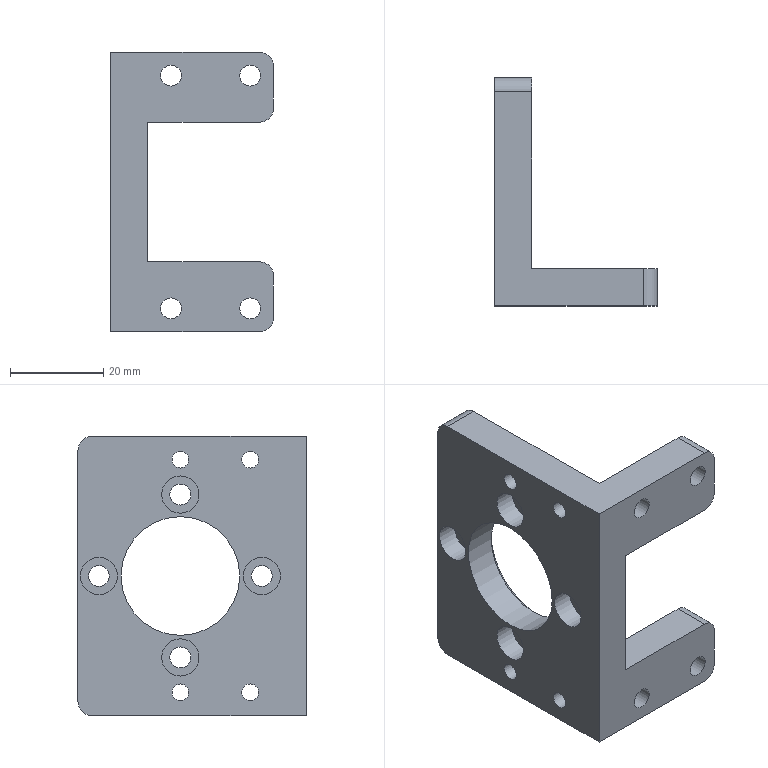Part | 1 solid | 56 faces | box 35 x 49 x 60 mm | volume 22926 mm3 | cylinder 31 | plane 24 | cone 1 | commonest cylinder face diameters 6 x10 4.5 x8 8 x8 3.6 x4 25.5 x1
STEP:
#1=CARTESIAN_POINT('',(4.6,12.,52.));
#2=VERTEX_POINT('',#1);
#3=CARTESIAN_POINT('',(4.6,12.,55.));
#4=DIRECTION('',(1.,0.,0.));
#5=DIRECTION('',(0.,0.,-1.));
#6=AXIS2_PLACEMENT_3D('',#3,#4,#5);
#7=CIRCLE('',#6,3.);
#8=EDGE_CURVE('',#2,#2,#7,.T.);
#9=ORIENTED_EDGE('',*,*,#8,.T.);
#10=EDGE_LOOP('',(#9));
#11=FACE_BOUND('',#10,.T.);
#12=CARTESIAN_POINT('',(4.6,12.,53.2));
#13=VERTEX_POINT('',#12);
#14=CARTESIAN_POINT('',(4.6,12.,55.));
#15=DIRECTION('',(1.,0.,0.));
#16=DIRECTION('',(0.,0.,-1.));
#17=AXIS2_PLACEMENT_3D('',#14,#15,#16);
#18=CIRCLE('',#17,1.8);
#19=EDGE_CURVE('',#13,#13,#18,.T.);
#20=ORIENTED_EDGE('',*,*,#19,.F.);
#21=EDGE_LOOP('',(#20));
#22=FACE_BOUND('',#21,.T.);
#23=CARTESIAN_POINT('',(4.6,13.8,55.));
#24=DIRECTION('',(-1.,0.,0.));
#25=DIRECTION('',(0.,0.,1.));
#26=AXIS2_PLACEMENT_3D('',#23,#24,#25);
#27=PLANE('',#26);
#28=ADVANCED_FACE('',(#11,#22),#27,.F.);
#29=CARTESIAN_POINT('',(4.6,12.,8.));
#30=VERTEX_POINT('',#29);
#31=CARTESIAN_POINT('',(4.6,12.,5.));
#32=DIRECTION('',(1.,0.,0.));
#33=DIRECTION('',(0.,0.,1.));
#34=AXIS2_PLACEMENT_3D('',#31,#32,#33);
#35=CIRCLE('',#34,3.);
#36=EDGE_CURVE('',#30,#30,#35,.T.);
#37=ORIENTED_EDGE('',*,*,#36,.T.);
#38=EDGE_LOOP('',(#37));
#39=FACE_BOUND('',#38,.T.);
#40=CARTESIAN_POINT('',(4.6,12.,6.8));
#41=VERTEX_POINT('',#40);
#42=CARTESIAN_POINT('',(4.6,12.,5.));
#43=DIRECTION('',(1.,0.,0.));
#44=DIRECTION('',(0.,0.,1.));
#45=AXIS2_PLACEMENT_3D('',#42,#43,#44);
#46=CIRCLE('',#45,1.8);
#47=EDGE_CURVE('',#41,#41,#46,.T.);
#48=ORIENTED_EDGE('',*,*,#47,.F.);
#49=EDGE_LOOP('',(#48));
#50=FACE_BOUND('',#49,.T.);
#51=CARTESIAN_POINT('',(4.6,13.8,55.));
#52=DIRECTION('',(-1.,0.,0.));
#53=DIRECTION('',(0.,0.,1.));
#54=AXIS2_PLACEMENT_3D('',#51,#52,#53);
#55=PLANE('',#54);
#56=ADVANCED_FACE('',(#39,#50),#55,.F.);
#57=CARTESIAN_POINT('',(4.6,27.,58.));
#58=VERTEX_POINT('',#57);
#59=CARTESIAN_POINT('',(4.6,27.,55.));
#60=DIRECTION('',(1.,0.,0.));
#61=DIRECTION('',(0.,0.,1.));
#62=AXIS2_PLACEMENT_3D('',#59,#60,#61);
#63=CIRCLE('',#62,3.);
#64=EDGE_CURVE('',#58,#58,#63,.T.);
#65=ORIENTED_EDGE('',*,*,#64,.T.);
#66=EDGE_LOOP('',(#65));
#67=FACE_BOUND('',#66,.T.);
#68=CARTESIAN_POINT('',(4.6,27.,56.8));
#69=VERTEX_POINT('',#68);
#70=CARTESIAN_POINT('',(4.6,27.,55.));
#71=DIRECTION('',(1.,0.,0.));
#72=DIRECTION('',(0.,0.,1.));
#73=AXIS2_PLACEMENT_3D('',#70,#71,#72);
#74=CIRCLE('',#73,1.8);
#75=EDGE_CURVE('',#69,#69,#74,.T.);
#76=ORIENTED_EDGE('',*,*,#75,.F.);
#77=EDGE_LOOP('',(#76));
#78=FACE_BOUND('',#77,.T.);
#79=CARTESIAN_POINT('',(4.6,13.8,55.));
#80=DIRECTION('',(-1.,0.,0.));
#81=DIRECTION('',(0.,0.,1.));
#82=AXIS2_PLACEMENT_3D('',#79,#80,#81);
#83=PLANE('',#82);
#84=ADVANCED_FACE('',(#67,#78),#83,.F.);
#85=CARTESIAN_POINT('',(4.6,27.,8.));
#86=VERTEX_POINT('',#85);
#87=CARTESIAN_POINT('',(4.6,27.,5.));
#88=DIRECTION('',(1.,0.,0.));
#89=DIRECTION('',(0.,0.,1.));
#90=AXIS2_PLACEMENT_3D('',#87,#88,#89);
#91=CIRCLE('',#90,3.);
#92=EDGE_CURVE('',#86,#86,#91,.T.);
#93=ORIENTED_EDGE('',*,*,#92,.T.);
#94=EDGE_LOOP('',(#93));
#95=FACE_BOUND('',#94,.T.);
#96=CARTESIAN_POINT('',(4.6,27.,6.8));
#97=VERTEX_POINT('',#96);
#98=CARTESIAN_POINT('',(4.6,27.,5.));
#99=DIRECTION('',(1.,0.,0.));
#100=DIRECTION('',(0.,0.,1.));
#101=AXIS2_PLACEMENT_3D('',#98,#99,#100);
#102=CIRCLE('',#101,1.8);
#103=EDGE_CURVE('',#97,#97,#102,.T.);
#104=ORIENTED_EDGE('',*,*,#103,.F.);
#105=EDGE_LOOP('',(#104));
#106=FACE_BOUND('',#105,.T.);
#107=CARTESIAN_POINT('',(4.6,13.8,55.));
#108=DIRECTION('',(-1.,0.,0.));
#109=DIRECTION('',(0.,0.,1.));
#110=AXIS2_PLACEMENT_3D('',#107,#108,#109);
#111=PLANE('',#110);
#112=ADVANCED_FACE('',(#95,#106),#111,.F.);
#113=CARTESIAN_POINT('',(13.,3.4,51.));
#114=VERTEX_POINT('',#113);
#115=CARTESIAN_POINT('',(13.,3.4,55.));
#116=DIRECTION('',(0.,1.,0.));
#117=DIRECTION('',(0.,0.,-1.));
#118=AXIS2_PLACEMENT_3D('',#115,#116,#117);
#119=CIRCLE('',#118,4.);
#120=EDGE_CURVE('',#114,#114,#119,.T.);
#121=ORIENTED_EDGE('',*,*,#120,.T.);
#122=EDGE_LOOP('',(#121));
#123=FACE_BOUND('',#122,.T.);
#124=CARTESIAN_POINT('',(13.,3.4,52.75));
#125=VERTEX_POINT('',#124);
#126=CARTESIAN_POINT('',(13.,3.4,55.));
#127=DIRECTION('',(0.,1.,0.));
#128=DIRECTION('',(0.,0.,-1.));
#129=AXIS2_PLACEMENT_3D('',#126,#127,#128);
#130=CIRCLE('',#129,2.25);
#131=EDGE_CURVE('',#125,#125,#130,.T.);
#132=ORIENTED_EDGE('',*,*,#131,.F.);
#133=EDGE_LOOP('',(#132));
#134=FACE_BOUND('',#133,.T.);
#135=CARTESIAN_POINT('',(32.25,3.4,5.));
#136=DIRECTION('',(0.,-1.,0.));
#137=DIRECTION('',(0.,0.,-1.));
#138=AXIS2_PLACEMENT_3D('',#135,#136,#137);
#139=PLANE('',#138);
#140=ADVANCED_FACE('',(#123,#134),#139,.F.);
#141=CARTESIAN_POINT('',(30.,3.4,51.));
#142=VERTEX_POINT('',#141);
#143=CARTESIAN_POINT('',(30.,3.4,55.));
#144=DIRECTION('',(0.,1.,0.));
#145=DIRECTION('',(0.,0.,-1.));
#146=AXIS2_PLACEMENT_3D('',#143,#144,#145);
#147=CIRCLE('',#146,4.);
#148=EDGE_CURVE('',#142,#142,#147,.T.);
#149=ORIENTED_EDGE('',*,*,#148,.T.);
#150=EDGE_LOOP('',(#149));
#151=FACE_BOUND('',#150,.T.);
#152=CARTESIAN_POINT('',(30.,3.4,52.75));
#153=VERTEX_POINT('',#152);
#154=CARTESIAN_POINT('',(30.,3.4,55.));
#155=DIRECTION('',(0.,1.,0.));
#156=DIRECTION('',(0.,0.,-1.));
#157=AXIS2_PLACEMENT_3D('',#154,#155,#156);
#158=CIRCLE('',#157,2.25);
#159=EDGE_CURVE('',#153,#153,#158,.T.);
#160=ORIENTED_EDGE('',*,*,#159,.F.);
#161=EDGE_LOOP('',(#160));
#162=FACE_BOUND('',#161,.T.);
#163=CARTESIAN_POINT('',(32.25,3.4,5.));
#164=DIRECTION('',(0.,-1.,0.));
#165=DIRECTION('',(0.,0.,-1.));
#166=AXIS2_PLACEMENT_3D('',#163,#164,#165);
#167=PLANE('',#166);
#168=ADVANCED_FACE('',(#151,#162),#167,.F.);
#169=CARTESIAN_POINT('',(13.,3.4,1.));
#170=VERTEX_POINT('',#169);
#171=CARTESIAN_POINT('',(13.,3.4,5.));
#172=DIRECTION('',(0.,1.,0.));
#173=DIRECTION('',(0.,0.,-1.));
#174=AXIS2_PLACEMENT_3D('',#171,#172,#173);
#175=CIRCLE('',#174,4.);
#176=EDGE_CURVE('',#170,#170,#175,.T.);
#177=ORIENTED_EDGE('',*,*,#176,.T.);
#178=EDGE_LOOP('',(#177));
#179=FACE_BOUND('',#178,.T.);
#180=CARTESIAN_POINT('',(13.,3.4,2.75));
#181=VERTEX_POINT('',#180);
#182=CARTESIAN_POINT('',(13.,3.4,5.));
#183=DIRECTION('',(0.,1.,0.));
#184=DIRECTION('',(0.,0.,-1.));
#185=AXIS2_PLACEMENT_3D('',#182,#183,#184);
#186=CIRCLE('',#185,2.25);
#187=EDGE_CURVE('',#181,#181,#186,.T.);
#188=ORIENTED_EDGE('',*,*,#187,.F.);
#189=EDGE_LOOP('',(#188));
#190=FACE_BOUND('',#189,.T.);
#191=CARTESIAN_POINT('',(32.25,3.4,5.));
#192=DIRECTION('',(0.,-1.,0.));
#193=DIRECTION('',(0.,0.,-1.));
#194=AXIS2_PLACEMENT_3D('',#191,#192,#193);
#195=PLANE('',#194);
#196=ADVANCED_FACE('',(#179,#190),#195,.F.);
#197=CARTESIAN_POINT('',(30.,3.4,9.));
#198=VERTEX_POINT('',#197);
#199=CARTESIAN_POINT('',(30.,3.4,5.));
#200=DIRECTION('',(0.,1.,0.));
#201=DIRECTION('',(0.,0.,1.));
#202=AXIS2_PLACEMENT_3D('',#199,#200,#201);
#203=CIRCLE('',#202,4.);
#204=EDGE_CURVE('',#198,#198,#203,.T.);
#205=ORIENTED_EDGE('',*,*,#204,.T.);
#206=EDGE_LOOP('',(#205));
#207=FACE_BOUND('',#206,.T.);
#208=CARTESIAN_POINT('',(30.,3.4,7.25));
#209=VERTEX_POINT('',#208);
#210=CARTESIAN_POINT('',(30.,3.4,5.));
#211=DIRECTION('',(0.,1.,0.));
#212=DIRECTION('',(0.,0.,1.));
#213=AXIS2_PLACEMENT_3D('',#210,#211,#212);
#214=CIRCLE('',#213,2.25);
#215=EDGE_CURVE('',#209,#209,#214,.T.);
#216=ORIENTED_EDGE('',*,*,#215,.F.);
#217=EDGE_LOOP('',(#216));
#218=FACE_BOUND('',#217,.T.);
#219=CARTESIAN_POINT('',(32.25,3.4,5.));
#220=DIRECTION('',(0.,-1.,0.));
#221=DIRECTION('',(0.,0.,-1.));
#222=AXIS2_PLACEMENT_3D('',#219,#220,#221);
#223=PLANE('',#222);
#224=ADVANCED_FACE('',(#207,#218),#223,.F.);
#225=CARTESIAN_POINT('',(35.,0.,12.));
#226=VERTEX_POINT('',#225);
#227=CARTESIAN_POINT('',(32.,0.,15.));
#228=VERTEX_POINT('',#227);
#229=CARTESIAN_POINT('',(32.,0.,12.));
#230=DIRECTION('',(0.,-1.,0.));
#231=DIRECTION('',(0.,0.,1.));
#232=AXIS2_PLACEMENT_3D('',#229,#230,#231);
#233=CIRCLE('',#232,3.);
#234=EDGE_CURVE('',#226,#228,#233,.T.);
#235=ORIENTED_EDGE('',*,*,#234,.F.);
#236=CARTESIAN_POINT('',(35.,8.,12.));
#237=VERTEX_POINT('',#236);
#238=CARTESIAN_POINT('',(35.,0.,12.));
#239=DIRECTION('',(0.,-1.,0.));
#240=VECTOR('',#239,1000.);
#241=LINE('',#238,#240);
#242=EDGE_CURVE('',#237,#226,#241,.T.);
#243=ORIENTED_EDGE('',*,*,#242,.F.);
#244=CARTESIAN_POINT('',(32.,8.,15.));
#245=VERTEX_POINT('',#244);
#246=CARTESIAN_POINT('',(32.,8.,12.));
#247=DIRECTION('',(0.,1.,0.));
#248=DIRECTION('',(1.,0.,0.));
#249=AXIS2_PLACEMENT_3D('',#246,#247,#248);
#250=CIRCLE('',#249,3.);
#251=EDGE_CURVE('',#245,#237,#250,.T.);
#252=ORIENTED_EDGE('',*,*,#251,.F.);
#253=CARTESIAN_POINT('',(32.,-2.,15.));
#254=DIRECTION('',(0.,1.,0.));
#255=VECTOR('',#254,1000.);
#256=LINE('',#253,#255);
#257=EDGE_CURVE('',#228,#245,#256,.T.);
#258=ORIENTED_EDGE('',*,*,#257,.F.);
#259=EDGE_LOOP('',(#235,#243,#252,#258));
#260=FACE_BOUND('',#259,.T.);
#261=CARTESIAN_POINT('',(32.,-2.,12.));
#262=DIRECTION('',(0.,1.,0.));
#263=DIRECTION('',(0.,0.,1.));
#264=AXIS2_PLACEMENT_3D('',#261,#262,#263);
#265=CYLINDRICAL_SURFACE('',#264,3.);
#266=ADVANCED_FACE('',(#260),#265,.T.);
#267=CARTESIAN_POINT('',(32.,0.,0.));
#268=VERTEX_POINT('',#267);
#269=CARTESIAN_POINT('',(35.,0.,3.));
#270=VERTEX_POINT('',#269);
#271=CARTESIAN_POINT('',(32.,0.,3.));
#272=DIRECTION('',(0.,-1.,0.));
#273=DIRECTION('',(0.,0.,1.));
#274=AXIS2_PLACEMENT_3D('',#271,#272,#273);
#275=CIRCLE('',#274,3.);
#276=EDGE_CURVE('',#268,#270,#275,.T.);
#277=ORIENTED_EDGE('',*,*,#276,.F.);
#278=CARTESIAN_POINT('',(32.,8.,0.));
#279=VERTEX_POINT('',#278);
#280=CARTESIAN_POINT('',(32.,0.,0.));
#281=DIRECTION('',(0.,-1.,0.));
#282=VECTOR('',#281,1000.);
#283=LINE('',#280,#282);
#284=EDGE_CURVE('',#279,#268,#283,.T.);
#285=ORIENTED_EDGE('',*,*,#284,.F.);
#286=CARTESIAN_POINT('',(35.,8.,3.));
#287=VERTEX_POINT('',#286);
#288=CARTESIAN_POINT('',(32.,8.,3.));
#289=DIRECTION('',(0.,1.,0.));
#290=DIRECTION('',(1.,0.,0.));
#291=AXIS2_PLACEMENT_3D('',#288,#289,#290);
#292=CIRCLE('',#291,3.);
#293=EDGE_CURVE('',#287,#279,#292,.T.);
#294=ORIENTED_EDGE('',*,*,#293,.F.);
#295=CARTESIAN_POINT('',(35.,0.,3.));
#296=DIRECTION('',(0.,1.,0.));
#297=VECTOR('',#296,1000.);
#298=LINE('',#295,#297);
#299=EDGE_CURVE('',#270,#287,#298,.T.);
#300=ORIENTED_EDGE('',*,*,#299,.F.);
#301=EDGE_LOOP('',(#277,#285,#294,#300));
#302=FACE_BOUND('',#301,.T.);
#303=CARTESIAN_POINT('',(32.,0.,3.));
#304=DIRECTION('',(0.,1.,0.));
#305=DIRECTION('',(0.,0.,1.));
#306=AXIS2_PLACEMENT_3D('',#303,#304,#305);
#307=CYLINDRICAL_SURFACE('',#306,3.);
#308=ADVANCED_FACE('',(#302),#307,.T.);
#309=CARTESIAN_POINT('',(32.,0.,45.));
#310=VERTEX_POINT('',#309);
#311=CARTESIAN_POINT('',(35.,0.,48.));
#312=VERTEX_POINT('',#311);
#313=CARTESIAN_POINT('',(32.,0.,48.));
#314=DIRECTION('',(0.,-1.,0.));
#315=DIRECTION('',(0.,0.,1.));
#316=AXIS2_PLACEMENT_3D('',#313,#314,#315);
#317=CIRCLE('',#316,3.);
#318=EDGE_CURVE('',#310,#312,#317,.T.);
#319=ORIENTED_EDGE('',*,*,#318,.F.);
#320=CARTESIAN_POINT('',(32.,8.,45.));
#321=VERTEX_POINT('',#320);
#322=CARTESIAN_POINT('',(32.,-2.,45.));
#323=DIRECTION('',(0.,-1.,0.));
#324=VECTOR('',#323,1000.);
#325=LINE('',#322,#324);
#326=EDGE_CURVE('',#321,#310,#325,.T.);
#327=ORIENTED_EDGE('',*,*,#326,.F.);
#328=CARTESIAN_POINT('',(35.,8.,48.));
#329=VERTEX_POINT('',#328);
#330=CARTESIAN_POINT('',(32.,8.,48.));
#331=DIRECTION('',(0.,1.,0.));
#332=DIRECTION('',(1.,0.,0.));
#333=AXIS2_PLACEMENT_3D('',#330,#331,#332);
#334=CIRCLE('',#333,3.);
#335=EDGE_CURVE('',#329,#321,#334,.T.);
#336=ORIENTED_EDGE('',*,*,#335,.F.);
#337=CARTESIAN_POINT('',(35.,0.,48.));
#338=DIRECTION('',(0.,1.,0.));
#339=VECTOR('',#338,1000.);
#340=LINE('',#337,#339);
#341=EDGE_CURVE('',#312,#329,#340,.T.);
#342=ORIENTED_EDGE('',*,*,#341,.F.);
#343=EDGE_LOOP('',(#319,#327,#336,#342));
#344=FACE_BOUND('',#343,.T.);
#345=CARTESIAN_POINT('',(32.,0.,48.));
#346=DIRECTION('',(0.,1.,0.));
#347=DIRECTION('',(0.,0.,1.));
#348=AXIS2_PLACEMENT_3D('',#345,#346,#347);
#349=CYLINDRICAL_SURFACE('',#348,3.);
#350=ADVANCED_FACE('',(#344),#349,.T.);
#351=CARTESIAN_POINT('',(35.,0.,57.));
#352=VERTEX_POINT('',#351);
#353=CARTESIAN_POINT('',(32.,0.,60.));
#354=VERTEX_POINT('',#353);
#355=CARTESIAN_POINT('',(32.,0.,57.));
#356=DIRECTION('',(0.,-1.,0.));
#357=DIRECTION('',(0.,0.,1.));
#358=AXIS2_PLACEMENT_3D('',#355,#356,#357);
#359=CIRCLE('',#358,3.);
#360=EDGE_CURVE('',#352,#354,#359,.T.);
#361=ORIENTED_EDGE('',*,*,#360,.F.);
#362=CARTESIAN_POINT('',(35.,8.,57.));
#363=VERTEX_POINT('',#362);
#364=CARTESIAN_POINT('',(35.,0.,57.));
#365=DIRECTION('',(0.,-1.,0.));
#366=VECTOR('',#365,1000.);
#367=LINE('',#364,#366);
#368=EDGE_CURVE('',#363,#352,#367,.T.);
#369=ORIENTED_EDGE('',*,*,#368,.F.);
#370=CARTESIAN_POINT('',(32.,8.,60.));
#371=VERTEX_POINT('',#370);
#372=CARTESIAN_POINT('',(32.,8.,57.));
#373=DIRECTION('',(0.,1.,0.));
#374=DIRECTION('',(1.,0.,0.));
#375=AXIS2_PLACEMENT_3D('',#372,#373,#374);
#376=CIRCLE('',#375,3.);
#377=EDGE_CURVE('',#371,#363,#376,.T.);
#378=ORIENTED_EDGE('',*,*,#377,.F.);
#379=CARTESIAN_POINT('',(32.,8.,60.));
#380=DIRECTION('',(0.,1.,0.));
#381=VECTOR('',#380,1000.);
#382=LINE('',#379,#381);
#383=EDGE_CURVE('',#354,#371,#382,.T.);
#384=ORIENTED_EDGE('',*,*,#383,.F.);
#385=EDGE_LOOP('',(#361,#369,#378,#384));
#386=FACE_BOUND('',#385,.T.);
#387=CARTESIAN_POINT('',(32.,0.,57.));
#388=DIRECTION('',(0.,-1.,0.));
#389=DIRECTION('',(0.,0.,-1.));
#390=AXIS2_PLACEMENT_3D('',#387,#388,#389);
#391=CYLINDRICAL_SURFACE('',#390,3.);
#392=ADVANCED_FACE('',(#386),#391,.T.);
#393=CARTESIAN_POINT('',(8.,49.,57.));
#394=VERTEX_POINT('',#393);
#395=CARTESIAN_POINT('',(8.,46.,60.));
#396=VERTEX_POINT('',#395);
#397=CARTESIAN_POINT('',(8.,46.,57.));
#398=DIRECTION('',(1.,0.,0.));
#399=DIRECTION('',(0.,0.,1.));
#400=AXIS2_PLACEMENT_3D('',#397,#398,#399);
#401=CIRCLE('',#400,3.);
#402=EDGE_CURVE('',#394,#396,#401,.T.);
#403=ORIENTED_EDGE('',*,*,#402,.F.);
#404=CARTESIAN_POINT('',(0.,49.,57.));
#405=VERTEX_POINT('',#404);
#406=CARTESIAN_POINT('',(8.,49.,57.));
#407=DIRECTION('',(1.,0.,0.));
#408=VECTOR('',#407,1000.);
#409=LINE('',#406,#408);
#410=EDGE_CURVE('',#405,#394,#409,.T.);
#411=ORIENTED_EDGE('',*,*,#410,.F.);
#412=CARTESIAN_POINT('',(0.,46.,60.));
#413=VERTEX_POINT('',#412);
#414=CARTESIAN_POINT('',(0.,46.,57.));
#415=DIRECTION('',(-1.,0.,0.));
#416=DIRECTION('',(0.,0.,-1.));
#417=AXIS2_PLACEMENT_3D('',#414,#415,#416);
#418=CIRCLE('',#417,3.);
#419=EDGE_CURVE('',#413,#405,#418,.T.);
#420=ORIENTED_EDGE('',*,*,#419,.F.);
#421=CARTESIAN_POINT('',(0.,46.,60.));
#422=DIRECTION('',(-1.,0.,0.));
#423=VECTOR('',#422,1000.);
#424=LINE('',#421,#423);
#425=EDGE_CURVE('',#396,#413,#424,.T.);
#426=ORIENTED_EDGE('',*,*,#425,.F.);
#427=EDGE_LOOP('',(#403,#411,#420,#426));
#428=FACE_BOUND('',#427,.T.);
#429=CARTESIAN_POINT('',(0.,46.,57.));
#430=DIRECTION('',(1.,0.,0.));
#431=DIRECTION('',(0.,0.,-1.));
#432=AXIS2_PLACEMENT_3D('',#429,#430,#431);
#433=CYLINDRICAL_SURFACE('',#432,3.);
#434=ADVANCED_FACE('',(#428),#433,.T.);
#435=CARTESIAN_POINT('',(8.,46.,0.));
#436=VERTEX_POINT('',#435);
#437=CARTESIAN_POINT('',(8.,49.,3.));
#438=VERTEX_POINT('',#437);
#439=CARTESIAN_POINT('',(8.,46.,3.));
#440=DIRECTION('',(1.,0.,0.));
#441=DIRECTION('',(0.,0.,1.));
#442=AXIS2_PLACEMENT_3D('',#439,#440,#441);
#443=CIRCLE('',#442,3.);
#444=EDGE_CURVE('',#436,#438,#443,.T.);
#445=ORIENTED_EDGE('',*,*,#444,.F.);
#446=CARTESIAN_POINT('',(0.,46.,0.));
#447=VERTEX_POINT('',#446);
#448=CARTESIAN_POINT('',(0.,46.,0.));
#449=DIRECTION('',(1.,0.,0.));
#450=VECTOR('',#449,1000.);
#451=LINE('',#448,#450);
#452=EDGE_CURVE('',#447,#436,#451,.T.);
#453=ORIENTED_EDGE('',*,*,#452,.F.);
#454=CARTESIAN_POINT('',(0.,49.,3.));
#455=VERTEX_POINT('',#454);
#456=CARTESIAN_POINT('',(0.,46.,3.));
#457=DIRECTION('',(-1.,0.,0.));
#458=DIRECTION('',(0.,0.,-1.));
#459=AXIS2_PLACEMENT_3D('',#456,#457,#458);
#460=CIRCLE('',#459,3.);
#461=EDGE_CURVE('',#455,#447,#460,.T.);
#462=ORIENTED_EDGE('',*,*,#461,.F.);
#463=CARTESIAN_POINT('',(8.,49.,3.));
#464=DIRECTION('',(-1.,0.,0.));
#465=VECTOR('',#464,1000.);
#466=LINE('',#463,#465);
#467=EDGE_CURVE('',#438,#455,#466,.T.);
#468=ORIENTED_EDGE('',*,*,#467,.F.);
#469=EDGE_LOOP('',(#445,#453,#462,#468));
#470=FACE_BOUND('',#469,.T.);
#471=CARTESIAN_POINT('',(8.,46.,3.));
#472=DIRECTION('',(-1.,0.,0.));
#473=DIRECTION('',(0.,0.,1.));
#474=AXIS2_PLACEMENT_3D('',#471,#472,#473);
#475=CYLINDRICAL_SURFACE('',#474,3.);
#476=ADVANCED_FACE('',(#470),#475,.T.);
#477=CARTESIAN_POINT('',(8.,0.,15.));
#478=VERTEX_POINT('',#477);
#479=CARTESIAN_POINT('',(0.,0.,15.));
#480=DIRECTION('',(-1.,0.,0.));
#481=VECTOR('',#480,1000.);
#482=LINE('',#479,#481);
#483=EDGE_CURVE('',#228,#478,#482,.T.);
#484=ORIENTED_EDGE('',*,*,#483,.F.);
#485=ORIENTED_EDGE('',*,*,#257,.T.);
#486=CARTESIAN_POINT('',(8.,8.,15.));
#487=VERTEX_POINT('',#486);
#488=CARTESIAN_POINT('',(8.,8.,15.));
#489=DIRECTION('',(-1.,0.,0.));
#490=VECTOR('',#489,1000.);
#491=LINE('',#488,#490);
#492=EDGE_CURVE('',#245,#487,#491,.T.);
#493=ORIENTED_EDGE('',*,*,#492,.T.);
#494=CARTESIAN_POINT('',(8.,-2.,15.));
#495=DIRECTION('',(0.,1.,0.));
#496=VECTOR('',#495,1000.);
#497=LINE('',#494,#496);
#498=EDGE_CURVE('',#478,#487,#497,.T.);
#499=ORIENTED_EDGE('',*,*,#498,.F.);
#500=EDGE_LOOP('',(#484,#485,#493,#499));
#501=FACE_BOUND('',#500,.T.);
#502=CARTESIAN_POINT('',(8.,-2.,15.));
#503=DIRECTION('',(0.,0.,-1.));
#504=DIRECTION('',(-1.,0.,0.));
#505=AXIS2_PLACEMENT_3D('',#502,#503,#504);
#506=PLANE('',#505);
#507=ADVANCED_FACE('',(#501),#506,.F.);
#508=CARTESIAN_POINT('',(8.,8.,45.));
#509=VERTEX_POINT('',#508);
#510=CARTESIAN_POINT('',(8.,8.,45.));
#511=DIRECTION('',(1.,0.,0.));
#512=VECTOR('',#511,1000.);
#513=LINE('',#510,#512);
#514=EDGE_CURVE('',#509,#321,#513,.T.);
#515=ORIENTED_EDGE('',*,*,#514,.T.);
#516=ORIENTED_EDGE('',*,*,#326,.T.);
#517=CARTESIAN_POINT('',(8.,0.,45.));
#518=VERTEX_POINT('',#517);
#519=CARTESIAN_POINT('',(0.,0.,45.));
#520=DIRECTION('',(1.,0.,0.));
#521=VECTOR('',#520,1000.);
#522=LINE('',#519,#521);
#523=EDGE_CURVE('',#518,#310,#522,.T.);
#524=ORIENTED_EDGE('',*,*,#523,.F.);
#525=CARTESIAN_POINT('',(8.,-2.,45.));
#526=DIRECTION('',(0.,1.,0.));
#527=VECTOR('',#526,1000.);
#528=LINE('',#525,#527);
#529=EDGE_CURVE('',#518,#509,#528,.T.);
#530=ORIENTED_EDGE('',*,*,#529,.T.);
#531=EDGE_LOOP('',(#515,#516,#524,#530));
#532=FACE_BOUND('',#531,.T.);
#533=CARTESIAN_POINT('',(8.,-2.,45.));
#534=DIRECTION('',(0.,0.,1.));
#535=DIRECTION('',(1.,0.,0.));
#536=AXIS2_PLACEMENT_3D('',#533,#534,#535);
#537=PLANE('',#536);
#538=ADVANCED_FACE('',(#532),#537,.F.);
#539=CARTESIAN_POINT('',(4.6,27.,51.5));
#540=VERTEX_POINT('',#539);
#541=CARTESIAN_POINT('',(4.6,27.,47.5));
#542=DIRECTION('',(-1.,0.,0.));
#543=DIRECTION('',(0.,0.,1.));
#544=AXIS2_PLACEMENT_3D('',#541,#542,#543);
#545=CIRCLE('',#544,4.);
#546=EDGE_CURVE('',#540,#540,#545,.T.);
#547=ORIENTED_EDGE('',*,*,#546,.T.);
#548=EDGE_LOOP('',(#547));
#549=FACE_BOUND('',#548,.T.);
#550=CARTESIAN_POINT('',(4.6,27.,49.75));
#551=VERTEX_POINT('',#550);
#552=CARTESIAN_POINT('',(4.6,27.,47.5));
#553=DIRECTION('',(-1.,0.,0.));
#554=DIRECTION('',(0.,0.,1.));
#555=AXIS2_PLACEMENT_3D('',#552,#553,#554);
#556=CIRCLE('',#555,2.25);
#557=EDGE_CURVE('',#551,#551,#556,.T.);
#558=ORIENTED_EDGE('',*,*,#557,.F.);
#559=EDGE_LOOP('',(#558));
#560=FACE_BOUND('',#559,.T.);
#561=CARTESIAN_POINT('',(4.6,13.8,55.));
#562=DIRECTION('',(-1.,0.,0.));
#563=DIRECTION('',(0.,0.,1.));
#564=AXIS2_PLACEMENT_3D('',#561,#562,#563);
#565=PLANE('',#564);
#566=ADVANCED_FACE('',(#549,#560),#565,.T.);
#567=CARTESIAN_POINT('',(4.6,27.,16.5));
#568=VERTEX_POINT('',#567);
#569=CARTESIAN_POINT('',(4.6,27.,12.5));
#570=DIRECTION('',(-1.,0.,0.));
#571=DIRECTION('',(0.,0.,1.));
#572=AXIS2_PLACEMENT_3D('',#569,#570,#571);
#573=CIRCLE('',#572,4.);
#574=EDGE_CURVE('',#568,#568,#573,.T.);
#575=ORIENTED_EDGE('',*,*,#574,.T.);
#576=EDGE_LOOP('',(#575));
#577=FACE_BOUND('',#576,.T.);
#578=CARTESIAN_POINT('',(4.6,27.,14.75));
#579=VERTEX_POINT('',#578);
#580=CARTESIAN_POINT('',(4.6,27.,12.5));
#581=DIRECTION('',(-1.,0.,0.));
#582=DIRECTION('',(0.,0.,1.));
#583=AXIS2_PLACEMENT_3D('',#580,#581,#582);
#584=CIRCLE('',#583,2.25);
#585=EDGE_CURVE('',#579,#579,#584,.T.);
#586=ORIENTED_EDGE('',*,*,#585,.F.);
#587=EDGE_LOOP('',(#586));
#588=FACE_BOUND('',#587,.T.);
#589=CARTESIAN_POINT('',(4.6,13.8,55.));
#590=DIRECTION('',(-1.,0.,0.));
#591=DIRECTION('',(0.,0.,1.));
#592=AXIS2_PLACEMENT_3D('',#589,#590,#591);
#593=PLANE('',#592);
#594=ADVANCED_FACE('',(#577,#588),#593,.T.);
#595=CARTESIAN_POINT('',(4.6,44.5,34.));
#596=VERTEX_POINT('',#595);
#597=CARTESIAN_POINT('',(4.6,44.5,30.));
#598=DIRECTION('',(-1.,0.,0.));
#599=DIRECTION('',(0.,0.,1.));
#600=AXIS2_PLACEMENT_3D('',#597,#598,#599);
#601=CIRCLE('',#600,4.);
#602=EDGE_CURVE('',#596,#596,#601,.T.);
#603=ORIENTED_EDGE('',*,*,#602,.T.);
#604=EDGE_LOOP('',(#603));
#605=FACE_BOUND('',#604,.T.);
#606=CARTESIAN_POINT('',(4.6,44.5,32.25));
#607=VERTEX_POINT('',#606);
#608=CARTESIAN_POINT('',(4.6,44.5,30.));
#609=DIRECTION('',(-1.,0.,0.));
#610=DIRECTION('',(0.,0.,1.));
#611=AXIS2_PLACEMENT_3D('',#608,#609,#610);
#612=CIRCLE('',#611,2.25);
#613=EDGE_CURVE('',#607,#607,#612,.T.);
#614=ORIENTED_EDGE('',*,*,#613,.F.);
#615=EDGE_LOOP('',(#614));
#616=FACE_BOUND('',#615,.T.);
#617=CARTESIAN_POINT('',(4.6,13.8,55.));
#618=DIRECTION('',(-1.,0.,0.));
#619=DIRECTION('',(0.,0.,1.));
#620=AXIS2_PLACEMENT_3D('',#617,#618,#619);
#621=PLANE('',#620);
#622=ADVANCED_FACE('',(#605,#616),#621,.T.);
#623=CARTESIAN_POINT('',(4.6,9.5,34.));
#624=VERTEX_POINT('',#623);
#625=CARTESIAN_POINT('',(4.6,9.5,30.));
#626=DIRECTION('',(-1.,0.,0.));
#627=DIRECTION('',(0.,0.,1.));
#628=AXIS2_PLACEMENT_3D('',#625,#626,#627);
#629=CIRCLE('',#628,4.);
#630=EDGE_CURVE('',#624,#624,#629,.T.);
#631=ORIENTED_EDGE('',*,*,#630,.T.);
#632=EDGE_LOOP('',(#631));
#633=FACE_BOUND('',#632,.T.);
#634=CARTESIAN_POINT('',(4.6,9.5,32.25));
#635=VERTEX_POINT('',#634);
#636=CARTESIAN_POINT('',(4.6,9.5,30.));
#637=DIRECTION('',(-1.,0.,0.));
#638=DIRECTION('',(0.,0.,1.));
#639=AXIS2_PLACEMENT_3D('',#636,#637,#638);
#640=CIRCLE('',#639,2.25);
#641=EDGE_CURVE('',#635,#635,#640,.T.);
#642=ORIENTED_EDGE('',*,*,#641,.F.);
#643=EDGE_LOOP('',(#642));
#644=FACE_BOUND('',#643,.T.);
#645=CARTESIAN_POINT('',(4.6,13.8,55.));
#646=DIRECTION('',(-1.,0.,0.));
#647=DIRECTION('',(0.,0.,1.));
#648=AXIS2_PLACEMENT_3D('',#645,#646,#647);
#649=PLANE('',#648);
#650=ADVANCED_FACE('',(#633,#644),#649,.T.);
#651=CARTESIAN_POINT('',(0.,0.,0.));
#652=VERTEX_POINT('',#651);
#653=CARTESIAN_POINT('',(0.,49.,0.));
#654=DIRECTION('',(0.,-1.,0.));
#655=VECTOR('',#654,1000.);
#656=LINE('',#653,#655);
#657=EDGE_CURVE('',#447,#652,#656,.T.);
#658=ORIENTED_EDGE('',*,*,#657,.F.);
#659=ORIENTED_EDGE('',*,*,#452,.T.);
#660=CARTESIAN_POINT('',(8.,8.,0.));
#661=VERTEX_POINT('',#660);
#662=CARTESIAN_POINT('',(8.,8.,0.));
#663=DIRECTION('',(0.,1.,0.));
#664=VECTOR('',#663,1000.);
#665=LINE('',#662,#664);
#666=EDGE_CURVE('',#661,#436,#665,.T.);
#667=ORIENTED_EDGE('',*,*,#666,.F.);
#668=CARTESIAN_POINT('',(35.,8.,0.));
#669=DIRECTION('',(-1.,0.,0.));
#670=VECTOR('',#669,1000.);
#671=LINE('',#668,#670);
#672=EDGE_CURVE('',#279,#661,#671,.T.);
#673=ORIENTED_EDGE('',*,*,#672,.F.);
#674=ORIENTED_EDGE('',*,*,#284,.T.);
#675=CARTESIAN_POINT('',(0.,0.,0.));
#676=DIRECTION('',(1.,0.,0.));
#677=VECTOR('',#676,1000.);
#678=LINE('',#675,#677);
#679=EDGE_CURVE('',#652,#268,#678,.T.);
#680=ORIENTED_EDGE('',*,*,#679,.F.);
#681=EDGE_LOOP('',(#658,#659,#667,#673,#674,#680));
#682=FACE_BOUND('',#681,.T.);
#683=CARTESIAN_POINT('',(0.,0.,0.));
#684=DIRECTION('',(0.,0.,1.));
#685=DIRECTION('',(1.,0.,0.));
#686=AXIS2_PLACEMENT_3D('',#683,#684,#685);
#687=PLANE('',#686);
#688=ADVANCED_FACE('',(#682),#687,.F.);
#689=CARTESIAN_POINT('',(8.,8.,60.));
#690=VERTEX_POINT('',#689);
#691=CARTESIAN_POINT('',(8.,8.,60.));
#692=DIRECTION('',(0.,1.,0.));
#693=VECTOR('',#692,1000.);
#694=LINE('',#691,#693);
#695=EDGE_CURVE('',#690,#396,#694,.T.);
#696=ORIENTED_EDGE('',*,*,#695,.T.);
#697=ORIENTED_EDGE('',*,*,#425,.T.);
#698=CARTESIAN_POINT('',(0.,0.,60.));
#699=VERTEX_POINT('',#698);
#700=CARTESIAN_POINT('',(0.,49.,60.));
#701=DIRECTION('',(0.,-1.,0.));
#702=VECTOR('',#701,1000.);
#703=LINE('',#700,#702);
#704=EDGE_CURVE('',#413,#699,#703,.T.);
#705=ORIENTED_EDGE('',*,*,#704,.T.);
#706=CARTESIAN_POINT('',(0.,0.,60.));
#707=DIRECTION('',(1.,0.,0.));
#708=VECTOR('',#707,1000.);
#709=LINE('',#706,#708);
#710=EDGE_CURVE('',#699,#354,#709,.T.);
#711=ORIENTED_EDGE('',*,*,#710,.T.);
#712=ORIENTED_EDGE('',*,*,#383,.T.);
#713=CARTESIAN_POINT('',(35.,8.,60.));
#714=DIRECTION('',(-1.,0.,0.));
#715=VECTOR('',#714,1000.);
#716=LINE('',#713,#715);
#717=EDGE_CURVE('',#371,#690,#716,.T.);
#718=ORIENTED_EDGE('',*,*,#717,.T.);
#719=EDGE_LOOP('',(#696,#697,#705,#711,#712,#718));
#720=FACE_BOUND('',#719,.T.);
#721=CARTESIAN_POINT('',(0.,0.,60.));
#722=DIRECTION('',(0.,0.,1.));
#723=DIRECTION('',(1.,0.,0.));
#724=AXIS2_PLACEMENT_3D('',#721,#722,#723);
#725=PLANE('',#724);
#726=ADVANCED_FACE('',(#720),#725,.T.);
#727=CARTESIAN_POINT('',(8.,9.5,32.25));
#728=VERTEX_POINT('',#727);
#729=CARTESIAN_POINT('',(8.,9.5,30.));
#730=DIRECTION('',(-1.,0.,0.));
#731=DIRECTION('',(0.,0.,1.));
#732=AXIS2_PLACEMENT_3D('',#729,#730,#731);
#733=CIRCLE('',#732,2.25);
#734=EDGE_CURVE('',#728,#728,#733,.T.);
#735=ORIENTED_EDGE('',*,*,#734,.T.);
#736=EDGE_LOOP('',(#735));
#737=FACE_BOUND('',#736,.T.);
#738=CARTESIAN_POINT('',(8.,44.5,32.25));
#739=VERTEX_POINT('',#738);
#740=CARTESIAN_POINT('',(8.,44.5,30.));
#741=DIRECTION('',(-1.,0.,0.));
#742=DIRECTION('',(0.,0.,1.));
#743=AXIS2_PLACEMENT_3D('',#740,#741,#742);
#744=CIRCLE('',#743,2.25);
#745=EDGE_CURVE('',#739,#739,#744,.T.);
#746=ORIENTED_EDGE('',*,*,#745,.T.);
#747=EDGE_LOOP('',(#746));
#748=FACE_BOUND('',#747,.T.);
#749=CARTESIAN_POINT('',(8.,27.,14.75));
#750=VERTEX_POINT('',#749);
#751=CARTESIAN_POINT('',(8.,27.,12.5));
#752=DIRECTION('',(-1.,0.,0.));
#753=DIRECTION('',(0.,0.,1.));
#754=AXIS2_PLACEMENT_3D('',#751,#752,#753);
#755=CIRCLE('',#754,2.25);
#756=EDGE_CURVE('',#750,#750,#755,.T.);
#757=ORIENTED_EDGE('',*,*,#756,.T.);
#758=EDGE_LOOP('',(#757));
#759=FACE_BOUND('',#758,.T.);
#760=CARTESIAN_POINT('',(8.,27.,49.75));
#761=VERTEX_POINT('',#760);
#762=CARTESIAN_POINT('',(8.,27.,47.5));
#763=DIRECTION('',(-1.,0.,0.));
#764=DIRECTION('',(0.,0.,1.));
#765=AXIS2_PLACEMENT_3D('',#762,#763,#764);
#766=CIRCLE('',#765,2.25);
#767=EDGE_CURVE('',#761,#761,#766,.T.);
#768=ORIENTED_EDGE('',*,*,#767,.T.);
#769=EDGE_LOOP('',(#768));
#770=FACE_BOUND('',#769,.T.);
#771=CARTESIAN_POINT('',(8.,27.,43.75));
#772=VERTEX_POINT('',#771);
#773=CARTESIAN_POINT('',(8.,27.,30.));
#774=DIRECTION('',(-1.,0.,0.));
#775=DIRECTION('',(0.,0.,1.));
#776=AXIS2_PLACEMENT_3D('',#773,#774,#775);
#777=CIRCLE('',#776,13.75);
#778=EDGE_CURVE('',#772,#772,#777,.T.);
#779=ORIENTED_EDGE('',*,*,#778,.T.);
#780=EDGE_LOOP('',(#779));
#781=FACE_BOUND('',#780,.T.);
#782=ORIENTED_EDGE('',*,*,#666,.T.);
#783=ORIENTED_EDGE('',*,*,#444,.T.);
#784=CARTESIAN_POINT('',(8.,49.,60.));
#785=DIRECTION('',(0.,0.,-1.));
#786=VECTOR('',#785,1000.);
#787=LINE('',#784,#786);
#788=EDGE_CURVE('',#394,#438,#787,.T.);
#789=ORIENTED_EDGE('',*,*,#788,.F.);
#790=ORIENTED_EDGE('',*,*,#402,.T.);
#791=ORIENTED_EDGE('',*,*,#695,.F.);
#792=CARTESIAN_POINT('',(8.,8.,60.));
#793=DIRECTION('',(0.,0.,-1.));
#794=VECTOR('',#793,1000.);
#795=LINE('',#792,#794);
#796=EDGE_CURVE('',#690,#509,#795,.T.);
#797=ORIENTED_EDGE('',*,*,#796,.T.);
#798=ORIENTED_EDGE('',*,*,#529,.F.);
#799=CARTESIAN_POINT('',(8.,0.,60.));
#800=DIRECTION('',(0.,0.,1.));
#801=VECTOR('',#800,1000.);
#802=LINE('',#799,#801);
#803=EDGE_CURVE('',#478,#518,#802,.T.);
#804=ORIENTED_EDGE('',*,*,#803,.F.);
#805=ORIENTED_EDGE('',*,*,#498,.T.);
#806=CARTESIAN_POINT('',(8.,8.,60.));
#807=DIRECTION('',(0.,0.,-1.));
#808=VECTOR('',#807,1000.);
#809=LINE('',#806,#808);
#810=EDGE_CURVE('',#487,#661,#809,.T.);
#811=ORIENTED_EDGE('',*,*,#810,.T.);
#812=EDGE_LOOP('',(#782,#783,#789,#790,#791,#797,#798,#804,#805,#811));
#813=FACE_BOUND('',#812,.T.);
#814=CARTESIAN_POINT('',(8.,27.,2.));
#815=VERTEX_POINT('',#814);
#816=CARTESIAN_POINT('',(8.,27.,5.));
#817=DIRECTION('',(1.,0.,0.));
#818=DIRECTION('',(0.,0.,-1.));
#819=AXIS2_PLACEMENT_3D('',#816,#817,#818);
#820=CIRCLE('',#819,3.);
#821=EDGE_CURVE('',#815,#815,#820,.T.);
#822=ORIENTED_EDGE('',*,*,#821,.F.);
#823=EDGE_LOOP('',(#822));
#824=FACE_BOUND('',#823,.T.);
#825=CARTESIAN_POINT('',(8.,27.,52.));
#826=VERTEX_POINT('',#825);
#827=CARTESIAN_POINT('',(8.,27.,55.));
#828=DIRECTION('',(1.,0.,0.));
#829=DIRECTION('',(0.,0.,-1.));
#830=AXIS2_PLACEMENT_3D('',#827,#828,#829);
#831=CIRCLE('',#830,3.);
#832=EDGE_CURVE('',#826,#826,#831,.T.);
#833=ORIENTED_EDGE('',*,*,#832,.F.);
#834=EDGE_LOOP('',(#833));
#835=FACE_BOUND('',#834,.T.);
#836=CARTESIAN_POINT('',(8.,12.,2.));
#837=VERTEX_POINT('',#836);
#838=CARTESIAN_POINT('',(8.,12.,5.));
#839=DIRECTION('',(1.,0.,0.));
#840=DIRECTION('',(0.,0.,-1.));
#841=AXIS2_PLACEMENT_3D('',#838,#839,#840);
#842=CIRCLE('',#841,3.);
#843=EDGE_CURVE('',#837,#837,#842,.T.);
#844=ORIENTED_EDGE('',*,*,#843,.F.);
#845=EDGE_LOOP('',(#844));
#846=FACE_BOUND('',#845,.T.);
#847=CARTESIAN_POINT('',(8.,12.,52.));
#848=VERTEX_POINT('',#847);
#849=CARTESIAN_POINT('',(8.,12.,55.));
#850=DIRECTION('',(1.,0.,0.));
#851=DIRECTION('',(0.,0.,-1.));
#852=AXIS2_PLACEMENT_3D('',#849,#850,#851);
#853=CIRCLE('',#852,3.);
#854=EDGE_CURVE('',#848,#848,#853,.T.);
#855=ORIENTED_EDGE('',*,*,#854,.F.);
#856=EDGE_LOOP('',(#855));
#857=FACE_BOUND('',#856,.T.);
#858=CARTESIAN_POINT('',(8.,8.,60.));
#859=DIRECTION('',(-1.,0.,0.));
#860=DIRECTION('',(0.,0.,1.));
#861=AXIS2_PLACEMENT_3D('',#858,#859,#860);
#862=PLANE('',#861);
#863=ADVANCED_FACE('',(#737,#748,#759,#770,#781,#813,#824,#835,#846,#857),#862,.F.);
#864=CARTESIAN_POINT('',(35.,8.,60.));
#865=DIRECTION('',(0.,0.,-1.));
#866=VECTOR('',#865,1000.);
#867=LINE('',#864,#866);
#868=EDGE_CURVE('',#237,#287,#867,.T.);
#869=ORIENTED_EDGE('',*,*,#868,.T.);
#870=ORIENTED_EDGE('',*,*,#293,.T.);
#871=ORIENTED_EDGE('',*,*,#672,.T.);
#872=ORIENTED_EDGE('',*,*,#810,.F.);
#873=ORIENTED_EDGE('',*,*,#492,.F.);
#874=ORIENTED_EDGE('',*,*,#251,.T.);
#875=EDGE_LOOP('',(#869,#870,#871,#872,#873,#874));
#876=FACE_BOUND('',#875,.T.);
#877=CARTESIAN_POINT('',(30.,8.,9.));
#878=VERTEX_POINT('',#877);
#879=CARTESIAN_POINT('',(30.,8.,5.));
#880=DIRECTION('',(0.,1.,0.));
#881=DIRECTION('',(0.,0.,1.));
#882=AXIS2_PLACEMENT_3D('',#879,#880,#881);
#883=CIRCLE('',#882,4.);
#884=EDGE_CURVE('',#878,#878,#883,.T.);
#885=ORIENTED_EDGE('',*,*,#884,.F.);
#886=EDGE_LOOP('',(#885));
#887=FACE_BOUND('',#886,.T.);
#888=CARTESIAN_POINT('',(13.,8.,9.));
#889=VERTEX_POINT('',#888);
#890=CARTESIAN_POINT('',(13.,8.,5.));
#891=DIRECTION('',(0.,1.,0.));
#892=DIRECTION('',(0.,0.,1.));
#893=AXIS2_PLACEMENT_3D('',#890,#891,#892);
#894=CIRCLE('',#893,4.);
#895=EDGE_CURVE('',#889,#889,#894,.T.);
#896=ORIENTED_EDGE('',*,*,#895,.F.);
#897=EDGE_LOOP('',(#896));
#898=FACE_BOUND('',#897,.T.);
#899=CARTESIAN_POINT('',(35.,8.,60.));
#900=DIRECTION('',(0.,-1.,0.));
#901=DIRECTION('',(1.,0.,0.));
#902=AXIS2_PLACEMENT_3D('',#899,#900,#901);
#903=PLANE('',#902);
#904=ADVANCED_FACE('',(#876,#887,#898),#903,.F.);
#905=CARTESIAN_POINT('',(35.,8.,60.));
#906=DIRECTION('',(0.,0.,-1.));
#907=VECTOR('',#906,1000.);
#908=LINE('',#905,#907);
#909=EDGE_CURVE('',#363,#329,#908,.T.);
#910=ORIENTED_EDGE('',*,*,#909,.F.);
#911=ORIENTED_EDGE('',*,*,#368,.T.);
#912=CARTESIAN_POINT('',(35.,0.,60.));
#913=DIRECTION('',(0.,0.,-1.));
#914=VECTOR('',#913,1000.);
#915=LINE('',#912,#914);
#916=EDGE_CURVE('',#352,#312,#915,.T.);
#917=ORIENTED_EDGE('',*,*,#916,.T.);
#918=ORIENTED_EDGE('',*,*,#341,.T.);
#919=EDGE_LOOP('',(#910,#911,#917,#918));
#920=FACE_BOUND('',#919,.T.);
#921=CARTESIAN_POINT('',(35.,0.,60.));
#922=DIRECTION('',(-1.,0.,0.));
#923=DIRECTION('',(0.,0.,1.));
#924=AXIS2_PLACEMENT_3D('',#921,#922,#923);
#925=PLANE('',#924);
#926=ADVANCED_FACE('',(#920),#925,.F.);
#927=ORIENTED_EDGE('',*,*,#916,.F.);
#928=ORIENTED_EDGE('',*,*,#360,.T.);
#929=ORIENTED_EDGE('',*,*,#710,.F.);
#930=CARTESIAN_POINT('',(0.,0.,60.));
#931=DIRECTION('',(0.,0.,-1.));
#932=VECTOR('',#931,1000.);
#933=LINE('',#930,#932);
#934=EDGE_CURVE('',#699,#652,#933,.T.);
#935=ORIENTED_EDGE('',*,*,#934,.T.);
#936=ORIENTED_EDGE('',*,*,#679,.T.);
#937=ORIENTED_EDGE('',*,*,#276,.T.);
#938=CARTESIAN_POINT('',(35.,0.,60.));
#939=DIRECTION('',(0.,0.,-1.));
#940=VECTOR('',#939,1000.);
#941=LINE('',#938,#940);
#942=EDGE_CURVE('',#226,#270,#941,.T.);
#943=ORIENTED_EDGE('',*,*,#942,.F.);
#944=ORIENTED_EDGE('',*,*,#234,.T.);
#945=ORIENTED_EDGE('',*,*,#483,.T.);
#946=ORIENTED_EDGE('',*,*,#803,.T.);
#947=ORIENTED_EDGE('',*,*,#523,.T.);
#948=ORIENTED_EDGE('',*,*,#318,.T.);
#949=EDGE_LOOP('',(#927,#928,#929,#935,#936,#937,#943,#944,#945,#946,#947,#948));
#950=FACE_BOUND('',#949,.T.);
#951=CARTESIAN_POINT('',(30.,0.,7.25));
#952=VERTEX_POINT('',#951);
#953=CARTESIAN_POINT('',(30.,0.,5.));
#954=DIRECTION('',(0.,1.,0.));
#955=DIRECTION('',(0.,0.,1.));
#956=AXIS2_PLACEMENT_3D('',#953,#954,#955);
#957=CIRCLE('',#956,2.25);
#958=EDGE_CURVE('',#952,#952,#957,.T.);
#959=ORIENTED_EDGE('',*,*,#958,.T.);
#960=EDGE_LOOP('',(#959));
#961=FACE_BOUND('',#960,.T.);
#962=CARTESIAN_POINT('',(13.,0.,7.25));
#963=VERTEX_POINT('',#962);
#964=CARTESIAN_POINT('',(13.,0.,5.));
#965=DIRECTION('',(0.,1.,0.));
#966=DIRECTION('',(0.,0.,1.));
#967=AXIS2_PLACEMENT_3D('',#964,#965,#966);
#968=CIRCLE('',#967,2.25);
#969=EDGE_CURVE('',#963,#963,#968,.T.);
#970=ORIENTED_EDGE('',*,*,#969,.T.);
#971=EDGE_LOOP('',(#970));
#972=FACE_BOUND('',#971,.T.);
#973=CARTESIAN_POINT('',(30.,0.,57.25));
#974=VERTEX_POINT('',#973);
#975=CARTESIAN_POINT('',(30.,0.,55.));
#976=DIRECTION('',(0.,1.,0.));
#977=DIRECTION('',(0.,0.,1.));
#978=AXIS2_PLACEMENT_3D('',#975,#976,#977);
#979=CIRCLE('',#978,2.25);
#980=EDGE_CURVE('',#974,#974,#979,.T.);
#981=ORIENTED_EDGE('',*,*,#980,.T.);
#982=EDGE_LOOP('',(#981));
#983=FACE_BOUND('',#982,.T.);
#984=CARTESIAN_POINT('',(13.,0.,57.25));
#985=VERTEX_POINT('',#984);
#986=CARTESIAN_POINT('',(13.,0.,55.));
#987=DIRECTION('',(0.,1.,0.));
#988=DIRECTION('',(0.,0.,1.));
#989=AXIS2_PLACEMENT_3D('',#986,#987,#988);
#990=CIRCLE('',#989,2.25);
#991=EDGE_CURVE('',#985,#985,#990,.T.);
#992=ORIENTED_EDGE('',*,*,#991,.T.);
#993=EDGE_LOOP('',(#992));
#994=FACE_BOUND('',#993,.T.);
#995=CARTESIAN_POINT('',(0.,0.,60.));
#996=DIRECTION('',(0.,1.,0.));
#997=DIRECTION('',(0.,0.,1.));
#998=AXIS2_PLACEMENT_3D('',#995,#996,#997);
#999=PLANE('',#998);
#1000=ADVANCED_FACE('',(#950,#961,#972,#983,#994),#999,.F.);
#1001=CARTESIAN_POINT('',(0.,49.,60.));
#1002=DIRECTION('',(0.,0.,-1.));
#1003=VECTOR('',#1002,1000.);
#1004=LINE('',#1001,#1003);
#1005=EDGE_CURVE('',#405,#455,#1004,.T.);
#1006=ORIENTED_EDGE('',*,*,#1005,.T.);
#1007=ORIENTED_EDGE('',*,*,#461,.T.);
#1008=ORIENTED_EDGE('',*,*,#657,.T.);
#1009=ORIENTED_EDGE('',*,*,#934,.F.);
#1010=ORIENTED_EDGE('',*,*,#704,.F.);
#1011=ORIENTED_EDGE('',*,*,#419,.T.);
#1012=EDGE_LOOP('',(#1006,#1007,#1008,#1009,#1010,#1011));
#1013=FACE_BOUND('',#1012,.T.);
#1014=CARTESIAN_POINT('',(0.,14.25,30.));
#1015=VERTEX_POINT('',#1014);
#1016=CARTESIAN_POINT('',(0.,27.,30.));
#1017=DIRECTION('',(-1.,0.,0.));
#1018=DIRECTION('',(0.,-1.,0.));
#1019=AXIS2_PLACEMENT_3D('',#1016,#1017,#1018);
#1020=CIRCLE('',#1019,12.75);
#1021=EDGE_CURVE('',#1015,#1015,#1020,.T.);
#1022=ORIENTED_EDGE('',*,*,#1021,.F.);
#1023=EDGE_LOOP('',(#1022));
#1024=FACE_BOUND('',#1023,.T.);
#1025=CARTESIAN_POINT('',(0.,9.5,34.));
#1026=VERTEX_POINT('',#1025);
#1027=CARTESIAN_POINT('',(0.,9.5,30.));
#1028=DIRECTION('',(-1.,0.,0.));
#1029=DIRECTION('',(0.,0.,1.));
#1030=AXIS2_PLACEMENT_3D('',#1027,#1028,#1029);
#1031=CIRCLE('',#1030,4.);
#1032=EDGE_CURVE('',#1026,#1026,#1031,.T.);
#1033=ORIENTED_EDGE('',*,*,#1032,.F.);
#1034=EDGE_LOOP('',(#1033));
#1035=FACE_BOUND('',#1034,.T.);
#1036=CARTESIAN_POINT('',(0.,44.5,34.));
#1037=VERTEX_POINT('',#1036);
#1038=CARTESIAN_POINT('',(0.,44.5,30.));
#1039=DIRECTION('',(-1.,0.,0.));
#1040=DIRECTION('',(0.,0.,1.));
#1041=AXIS2_PLACEMENT_3D('',#1038,#1039,#1040);
#1042=CIRCLE('',#1041,4.);
#1043=EDGE_CURVE('',#1037,#1037,#1042,.T.);
#1044=ORIENTED_EDGE('',*,*,#1043,.F.);
#1045=EDGE_LOOP('',(#1044));
#1046=FACE_BOUND('',#1045,.T.);
#1047=CARTESIAN_POINT('',(0.,27.,16.5));
#1048=VERTEX_POINT('',#1047);
#1049=CARTESIAN_POINT('',(0.,27.,12.5));
#1050=DIRECTION('',(-1.,0.,0.));
#1051=DIRECTION('',(0.,0.,1.));
#1052=AXIS2_PLACEMENT_3D('',#1049,#1050,#1051);
#1053=CIRCLE('',#1052,4.);
#1054=EDGE_CURVE('',#1048,#1048,#1053,.T.);
#1055=ORIENTED_EDGE('',*,*,#1054,.F.);
#1056=EDGE_LOOP('',(#1055));
#1057=FACE_BOUND('',#1056,.T.);
#1058=CARTESIAN_POINT('',(0.,27.,51.5));
#1059=VERTEX_POINT('',#1058);
#1060=CARTESIAN_POINT('',(0.,27.,47.5));
#1061=DIRECTION('',(-1.,0.,0.));
#1062=DIRECTION('',(0.,0.,1.));
#1063=AXIS2_PLACEMENT_3D('',#1060,#1061,#1062);
#1064=CIRCLE('',#1063,4.);
#1065=EDGE_CURVE('',#1059,#1059,#1064,.T.);
#1066=ORIENTED_EDGE('',*,*,#1065,.F.);
#1067=EDGE_LOOP('',(#1066));
#1068=FACE_BOUND('',#1067,.T.);
#1069=CARTESIAN_POINT('',(0.,27.,3.2));
#1070=VERTEX_POINT('',#1069);
#1071=CARTESIAN_POINT('',(0.,27.,5.));
#1072=DIRECTION('',(1.,0.,0.));
#1073=DIRECTION('',(0.,0.,-1.));
#1074=AXIS2_PLACEMENT_3D('',#1071,#1072,#1073);
#1075=CIRCLE('',#1074,1.8);
#1076=EDGE_CURVE('',#1070,#1070,#1075,.T.);
#1077=ORIENTED_EDGE('',*,*,#1076,.T.);
#1078=EDGE_LOOP('',(#1077));
#1079=FACE_BOUND('',#1078,.T.);
#1080=CARTESIAN_POINT('',(0.,27.,53.2));
#1081=VERTEX_POINT('',#1080);
#1082=CARTESIAN_POINT('',(0.,27.,55.));
#1083=DIRECTION('',(1.,0.,0.));
#1084=DIRECTION('',(0.,0.,-1.));
#1085=AXIS2_PLACEMENT_3D('',#1082,#1083,#1084);
#1086=CIRCLE('',#1085,1.8);
#1087=EDGE_CURVE('',#1081,#1081,#1086,.T.);
#1088=ORIENTED_EDGE('',*,*,#1087,.T.);
#1089=EDGE_LOOP('',(#1088));
#1090=FACE_BOUND('',#1089,.T.);
#1091=CARTESIAN_POINT('',(0.,12.,3.2));
#1092=VERTEX_POINT('',#1091);
#1093=CARTESIAN_POINT('',(0.,12.,5.));
#1094=DIRECTION('',(1.,0.,0.));
#1095=DIRECTION('',(0.,0.,-1.));
#1096=AXIS2_PLACEMENT_3D('',#1093,#1094,#1095);
#1097=CIRCLE('',#1096,1.8);
#1098=EDGE_CURVE('',#1092,#1092,#1097,.T.);
#1099=ORIENTED_EDGE('',*,*,#1098,.T.);
#1100=EDGE_LOOP('',(#1099));
#1101=FACE_BOUND('',#1100,.T.);
#1102=CARTESIAN_POINT('',(0.,12.,53.2));
#1103=VERTEX_POINT('',#1102);
#1104=CARTESIAN_POINT('',(0.,12.,55.));
#1105=DIRECTION('',(1.,0.,0.));
#1106=DIRECTION('',(0.,0.,-1.));
#1107=AXIS2_PLACEMENT_3D('',#1104,#1105,#1106);
#1108=CIRCLE('',#1107,1.8);
#1109=EDGE_CURVE('',#1103,#1103,#1108,.T.);
#1110=ORIENTED_EDGE('',*,*,#1109,.T.);
#1111=EDGE_LOOP('',(#1110));
#1112=FACE_BOUND('',#1111,.T.);
#1113=CARTESIAN_POINT('',(0.,49.,60.));
#1114=DIRECTION('',(1.,0.,0.));
#1115=DIRECTION('',(0.,0.,-1.));
#1116=AXIS2_PLACEMENT_3D('',#1113,#1114,#1115);
#1117=PLANE('',#1116);
#1118=ADVANCED_FACE('',(#1013,#1024,#1035,#1046,#1057,#1068,#1079,#1090,#1101,#1112),#1117,.F.);
#1119=ORIENTED_EDGE('',*,*,#788,.T.);
#1120=ORIENTED_EDGE('',*,*,#467,.T.);
#1121=ORIENTED_EDGE('',*,*,#1005,.F.);
#1122=ORIENTED_EDGE('',*,*,#410,.T.);
#1123=EDGE_LOOP('',(#1119,#1120,#1121,#1122));
#1124=FACE_BOUND('',#1123,.T.);
#1125=CARTESIAN_POINT('',(8.,49.,60.));
#1126=DIRECTION('',(0.,-1.,0.));
#1127=DIRECTION('',(0.,0.,-1.));
#1128=AXIS2_PLACEMENT_3D('',#1125,#1126,#1127);
#1129=PLANE('',#1128);
#1130=ADVANCED_FACE('',(#1124),#1129,.F.);
#1131=ORIENTED_EDGE('',*,*,#717,.F.);
#1132=ORIENTED_EDGE('',*,*,#377,.T.);
#1133=ORIENTED_EDGE('',*,*,#909,.T.);
#1134=ORIENTED_EDGE('',*,*,#335,.T.);
#1135=ORIENTED_EDGE('',*,*,#514,.F.);
#1136=ORIENTED_EDGE('',*,*,#796,.F.);
#1137=EDGE_LOOP('',(#1131,#1132,#1133,#1134,#1135,#1136));
#1138=FACE_BOUND('',#1137,.T.);
#1139=CARTESIAN_POINT('',(30.,8.,59.));
#1140=VERTEX_POINT('',#1139);
#1141=CARTESIAN_POINT('',(30.,8.,55.));
#1142=DIRECTION('',(0.,1.,0.));
#1143=DIRECTION('',(0.,0.,1.));
#1144=AXIS2_PLACEMENT_3D('',#1141,#1142,#1143);
#1145=CIRCLE('',#1144,4.);
#1146=EDGE_CURVE('',#1140,#1140,#1145,.T.);
#1147=ORIENTED_EDGE('',*,*,#1146,.F.);
#1148=EDGE_LOOP('',(#1147));
#1149=FACE_BOUND('',#1148,.T.);
#1150=CARTESIAN_POINT('',(13.,8.,59.));
#1151=VERTEX_POINT('',#1150);
#1152=CARTESIAN_POINT('',(13.,8.,55.));
#1153=DIRECTION('',(0.,1.,0.));
#1154=DIRECTION('',(0.,0.,1.));
#1155=AXIS2_PLACEMENT_3D('',#1152,#1153,#1154);
#1156=CIRCLE('',#1155,4.);
#1157=EDGE_CURVE('',#1151,#1151,#1156,.T.);
#1158=ORIENTED_EDGE('',*,*,#1157,.F.);
#1159=EDGE_LOOP('',(#1158));
#1160=FACE_BOUND('',#1159,.T.);
#1161=CARTESIAN_POINT('',(35.,8.,60.));
#1162=DIRECTION('',(0.,-1.,0.));
#1163=DIRECTION('',(1.,0.,0.));
#1164=AXIS2_PLACEMENT_3D('',#1161,#1162,#1163);
#1165=PLANE('',#1164);
#1166=ADVANCED_FACE('',(#1138,#1149,#1160),#1165,.F.);
#1167=ORIENTED_EDGE('',*,*,#942,.T.);
#1168=ORIENTED_EDGE('',*,*,#299,.T.);
#1169=ORIENTED_EDGE('',*,*,#868,.F.);
#1170=ORIENTED_EDGE('',*,*,#242,.T.);
#1171=EDGE_LOOP('',(#1167,#1168,#1169,#1170));
#1172=FACE_BOUND('',#1171,.T.);
#1173=CARTESIAN_POINT('',(35.,0.,60.));
#1174=DIRECTION('',(-1.,0.,0.));
#1175=DIRECTION('',(0.,0.,1.));
#1176=AXIS2_PLACEMENT_3D('',#1173,#1174,#1175);
#1177=PLANE('',#1176);
#1178=ADVANCED_FACE('',(#1172),#1177,.F.);
#1179=ORIENTED_EDGE('',*,*,#1021,.T.);
#1180=EDGE_LOOP('',(#1179));
#1181=FACE_BOUND('',#1180,.T.);
#1182=CARTESIAN_POINT('',(7.,27.,42.75));
#1183=VERTEX_POINT('',#1182);
#1184=CARTESIAN_POINT('',(7.,27.,30.));
#1185=DIRECTION('',(1.,0.,0.));
#1186=DIRECTION('',(0.,0.,1.));
#1187=AXIS2_PLACEMENT_3D('',#1184,#1185,#1186);
#1188=CIRCLE('',#1187,12.75);
#1189=EDGE_CURVE('',#1183,#1183,#1188,.T.);
#1190=ORIENTED_EDGE('',*,*,#1189,.T.);
#1191=EDGE_LOOP('',(#1190));
#1192=FACE_BOUND('',#1191,.T.);
#1193=CARTESIAN_POINT('',(45.,27.,30.));
#1194=DIRECTION('',(-1.,0.,0.));
#1195=DIRECTION('',(0.,-1.,0.));
#1196=AXIS2_PLACEMENT_3D('',#1193,#1194,#1195);
#1197=CYLINDRICAL_SURFACE('',#1196,12.75);
#1198=ADVANCED_FACE('',(#1181,#1192),#1197,.F.);
#1199=ORIENTED_EDGE('',*,*,#734,.F.);
#1200=EDGE_LOOP('',(#1199));
#1201=FACE_BOUND('',#1200,.T.);
#1202=ORIENTED_EDGE('',*,*,#641,.T.);
#1203=EDGE_LOOP('',(#1202));
#1204=FACE_BOUND('',#1203,.T.);
#1205=CARTESIAN_POINT('',(0.,9.5,30.));
#1206=DIRECTION('',(-1.,0.,0.));
#1207=DIRECTION('',(0.,0.,1.));
#1208=AXIS2_PLACEMENT_3D('',#1205,#1206,#1207);
#1209=CYLINDRICAL_SURFACE('',#1208,2.25);
#1210=ADVANCED_FACE('',(#1201,#1204),#1209,.F.);
#1211=ORIENTED_EDGE('',*,*,#630,.F.);
#1212=EDGE_LOOP('',(#1211));
#1213=FACE_BOUND('',#1212,.T.);
#1214=ORIENTED_EDGE('',*,*,#1032,.T.);
#1215=EDGE_LOOP('',(#1214));
#1216=FACE_BOUND('',#1215,.T.);
#1217=CARTESIAN_POINT('',(0.,9.5,30.));
#1218=DIRECTION('',(-1.,0.,0.));
#1219=DIRECTION('',(0.,0.,1.));
#1220=AXIS2_PLACEMENT_3D('',#1217,#1218,#1219);
#1221=CYLINDRICAL_SURFACE('',#1220,4.);
#1222=ADVANCED_FACE('',(#1213,#1216),#1221,.F.);
#1223=ORIENTED_EDGE('',*,*,#745,.F.);
#1224=EDGE_LOOP('',(#1223));
#1225=FACE_BOUND('',#1224,.T.);
#1226=ORIENTED_EDGE('',*,*,#613,.T.);
#1227=EDGE_LOOP('',(#1226));
#1228=FACE_BOUND('',#1227,.T.);
#1229=CARTESIAN_POINT('',(0.,44.5,30.));
#1230=DIRECTION('',(-1.,0.,0.));
#1231=DIRECTION('',(0.,0.,1.));
#1232=AXIS2_PLACEMENT_3D('',#1229,#1230,#1231);
#1233=CYLINDRICAL_SURFACE('',#1232,2.25);
#1234=ADVANCED_FACE('',(#1225,#1228),#1233,.F.);
#1235=ORIENTED_EDGE('',*,*,#602,.F.);
#1236=EDGE_LOOP('',(#1235));
#1237=FACE_BOUND('',#1236,.T.);
#1238=ORIENTED_EDGE('',*,*,#1043,.T.);
#1239=EDGE_LOOP('',(#1238));
#1240=FACE_BOUND('',#1239,.T.);
#1241=CARTESIAN_POINT('',(0.,44.5,30.));
#1242=DIRECTION('',(-1.,0.,0.));
#1243=DIRECTION('',(0.,0.,1.));
#1244=AXIS2_PLACEMENT_3D('',#1241,#1242,#1243);
#1245=CYLINDRICAL_SURFACE('',#1244,4.);
#1246=ADVANCED_FACE('',(#1237,#1240),#1245,.F.);
#1247=ORIENTED_EDGE('',*,*,#756,.F.);
#1248=EDGE_LOOP('',(#1247));
#1249=FACE_BOUND('',#1248,.T.);
#1250=ORIENTED_EDGE('',*,*,#585,.T.);
#1251=EDGE_LOOP('',(#1250));
#1252=FACE_BOUND('',#1251,.T.);
#1253=CARTESIAN_POINT('',(0.,27.,12.5));
#1254=DIRECTION('',(-1.,0.,0.));
#1255=DIRECTION('',(0.,0.,1.));
#1256=AXIS2_PLACEMENT_3D('',#1253,#1254,#1255);
#1257=CYLINDRICAL_SURFACE('',#1256,2.25);
#1258=ADVANCED_FACE('',(#1249,#1252),#1257,.F.);
#1259=ORIENTED_EDGE('',*,*,#574,.F.);
#1260=EDGE_LOOP('',(#1259));
#1261=FACE_BOUND('',#1260,.T.);
#1262=ORIENTED_EDGE('',*,*,#1054,.T.);
#1263=EDGE_LOOP('',(#1262));
#1264=FACE_BOUND('',#1263,.T.);
#1265=CARTESIAN_POINT('',(0.,27.,12.5));
#1266=DIRECTION('',(-1.,0.,0.));
#1267=DIRECTION('',(0.,0.,1.));
#1268=AXIS2_PLACEMENT_3D('',#1265,#1266,#1267);
#1269=CYLINDRICAL_SURFACE('',#1268,4.);
#1270=ADVANCED_FACE('',(#1261,#1264),#1269,.F.);
#1271=ORIENTED_EDGE('',*,*,#767,.F.);
#1272=EDGE_LOOP('',(#1271));
#1273=FACE_BOUND('',#1272,.T.);
#1274=ORIENTED_EDGE('',*,*,#557,.T.);
#1275=EDGE_LOOP('',(#1274));
#1276=FACE_BOUND('',#1275,.T.);
#1277=CARTESIAN_POINT('',(0.,27.,47.5));
#1278=DIRECTION('',(-1.,0.,0.));
#1279=DIRECTION('',(0.,0.,1.));
#1280=AXIS2_PLACEMENT_3D('',#1277,#1278,#1279);
#1281=CYLINDRICAL_SURFACE('',#1280,2.25);
#1282=ADVANCED_FACE('',(#1273,#1276),#1281,.F.);
#1283=ORIENTED_EDGE('',*,*,#546,.F.);
#1284=EDGE_LOOP('',(#1283));
#1285=FACE_BOUND('',#1284,.T.);
#1286=ORIENTED_EDGE('',*,*,#1065,.T.);
#1287=EDGE_LOOP('',(#1286));
#1288=FACE_BOUND('',#1287,.T.);
#1289=CARTESIAN_POINT('',(0.,27.,47.5));
#1290=DIRECTION('',(-1.,0.,0.));
#1291=DIRECTION('',(0.,0.,1.));
#1292=AXIS2_PLACEMENT_3D('',#1289,#1290,#1291);
#1293=CYLINDRICAL_SURFACE('',#1292,4.);
#1294=ADVANCED_FACE('',(#1285,#1288),#1293,.F.);
#1295=ORIENTED_EDGE('',*,*,#778,.F.);
#1296=EDGE_LOOP('',(#1295));
#1297=FACE_BOUND('',#1296,.T.);
#1298=ORIENTED_EDGE('',*,*,#1189,.F.);
#1299=EDGE_LOOP('',(#1298));
#1300=FACE_BOUND('',#1299,.T.);
#1301=CARTESIAN_POINT('',(8.,27.,30.));
#1302=DIRECTION('',(1.,0.,0.));
#1303=DIRECTION('',(0.,0.,-1.));
#1304=AXIS2_PLACEMENT_3D('',#1301,#1302,#1303);
#1305=CONICAL_SURFACE('',#1304,13.75,0.7854);
#1306=ADVANCED_FACE('',(#1297,#1300),#1305,.F.);
#1307=ORIENTED_EDGE('',*,*,#958,.F.);
#1308=EDGE_LOOP('',(#1307));
#1309=FACE_BOUND('',#1308,.T.);
#1310=ORIENTED_EDGE('',*,*,#215,.T.);
#1311=EDGE_LOOP('',(#1310));
#1312=FACE_BOUND('',#1311,.T.);
#1313=CARTESIAN_POINT('',(30.,8.,5.));
#1314=DIRECTION('',(0.,1.,0.));
#1315=DIRECTION('',(0.,0.,1.));
#1316=AXIS2_PLACEMENT_3D('',#1313,#1314,#1315);
#1317=CYLINDRICAL_SURFACE('',#1316,2.25);
#1318=ADVANCED_FACE('',(#1309,#1312),#1317,.F.);
#1319=ORIENTED_EDGE('',*,*,#204,.F.);
#1320=EDGE_LOOP('',(#1319));
#1321=FACE_BOUND('',#1320,.T.);
#1322=ORIENTED_EDGE('',*,*,#884,.T.);
#1323=EDGE_LOOP('',(#1322));
#1324=FACE_BOUND('',#1323,.T.);
#1325=CARTESIAN_POINT('',(30.,8.,5.));
#1326=DIRECTION('',(0.,1.,0.));
#1327=DIRECTION('',(0.,0.,1.));
#1328=AXIS2_PLACEMENT_3D('',#1325,#1326,#1327);
#1329=CYLINDRICAL_SURFACE('',#1328,4.);
#1330=ADVANCED_FACE('',(#1321,#1324),#1329,.F.);
#1331=ORIENTED_EDGE('',*,*,#969,.F.);
#1332=EDGE_LOOP('',(#1331));
#1333=FACE_BOUND('',#1332,.T.);
#1334=ORIENTED_EDGE('',*,*,#187,.T.);
#1335=EDGE_LOOP('',(#1334));
#1336=FACE_BOUND('',#1335,.T.);
#1337=CARTESIAN_POINT('',(13.,8.,5.));
#1338=DIRECTION('',(0.,1.,0.));
#1339=DIRECTION('',(0.,0.,1.));
#1340=AXIS2_PLACEMENT_3D('',#1337,#1338,#1339);
#1341=CYLINDRICAL_SURFACE('',#1340,2.25);
#1342=ADVANCED_FACE('',(#1333,#1336),#1341,.F.);
#1343=ORIENTED_EDGE('',*,*,#176,.F.);
#1344=EDGE_LOOP('',(#1343));
#1345=FACE_BOUND('',#1344,.T.);
#1346=ORIENTED_EDGE('',*,*,#895,.T.);
#1347=EDGE_LOOP('',(#1346));
#1348=FACE_BOUND('',#1347,.T.);
#1349=CARTESIAN_POINT('',(13.,8.,5.));
#1350=DIRECTION('',(0.,1.,0.));
#1351=DIRECTION('',(0.,0.,1.));
#1352=AXIS2_PLACEMENT_3D('',#1349,#1350,#1351);
#1353=CYLINDRICAL_SURFACE('',#1352,4.);
#1354=ADVANCED_FACE('',(#1345,#1348),#1353,.F.);
#1355=ORIENTED_EDGE('',*,*,#980,.F.);
#1356=EDGE_LOOP('',(#1355));
#1357=FACE_BOUND('',#1356,.T.);
#1358=ORIENTED_EDGE('',*,*,#159,.T.);
#1359=EDGE_LOOP('',(#1358));
#1360=FACE_BOUND('',#1359,.T.);
#1361=CARTESIAN_POINT('',(30.,8.,55.));
#1362=DIRECTION('',(0.,1.,0.));
#1363=DIRECTION('',(0.,0.,1.));
#1364=AXIS2_PLACEMENT_3D('',#1361,#1362,#1363);
#1365=CYLINDRICAL_SURFACE('',#1364,2.25);
#1366=ADVANCED_FACE('',(#1357,#1360),#1365,.F.);
#1367=ORIENTED_EDGE('',*,*,#148,.F.);
#1368=EDGE_LOOP('',(#1367));
#1369=FACE_BOUND('',#1368,.T.);
#1370=ORIENTED_EDGE('',*,*,#1146,.T.);
#1371=EDGE_LOOP('',(#1370));
#1372=FACE_BOUND('',#1371,.T.);
#1373=CARTESIAN_POINT('',(30.,8.,55.));
#1374=DIRECTION('',(0.,1.,0.));
#1375=DIRECTION('',(0.,0.,1.));
#1376=AXIS2_PLACEMENT_3D('',#1373,#1374,#1375);
#1377=CYLINDRICAL_SURFACE('',#1376,4.);
#1378=ADVANCED_FACE('',(#1369,#1372),#1377,.F.);
#1379=ORIENTED_EDGE('',*,*,#991,.F.);
#1380=EDGE_LOOP('',(#1379));
#1381=FACE_BOUND('',#1380,.T.);
#1382=ORIENTED_EDGE('',*,*,#131,.T.);
#1383=EDGE_LOOP('',(#1382));
#1384=FACE_BOUND('',#1383,.T.);
#1385=CARTESIAN_POINT('',(13.,8.,55.));
#1386=DIRECTION('',(0.,1.,0.));
#1387=DIRECTION('',(0.,0.,1.));
#1388=AXIS2_PLACEMENT_3D('',#1385,#1386,#1387);
#1389=CYLINDRICAL_SURFACE('',#1388,2.25);
#1390=ADVANCED_FACE('',(#1381,#1384),#1389,.F.);
#1391=ORIENTED_EDGE('',*,*,#120,.F.);
#1392=EDGE_LOOP('',(#1391));
#1393=FACE_BOUND('',#1392,.T.);
#1394=ORIENTED_EDGE('',*,*,#1157,.T.);
#1395=EDGE_LOOP('',(#1394));
#1396=FACE_BOUND('',#1395,.T.);
#1397=CARTESIAN_POINT('',(13.,8.,55.));
#1398=DIRECTION('',(0.,1.,0.));
#1399=DIRECTION('',(0.,0.,1.));
#1400=AXIS2_PLACEMENT_3D('',#1397,#1398,#1399);
#1401=CYLINDRICAL_SURFACE('',#1400,4.);
#1402=ADVANCED_FACE('',(#1393,#1396),#1401,.F.);
#1403=ORIENTED_EDGE('',*,*,#103,.T.);
#1404=EDGE_LOOP('',(#1403));
#1405=FACE_BOUND('',#1404,.T.);
#1406=ORIENTED_EDGE('',*,*,#1076,.F.);
#1407=EDGE_LOOP('',(#1406));
#1408=FACE_BOUND('',#1407,.T.);
#1409=CARTESIAN_POINT('',(8.,27.,5.));
#1410=DIRECTION('',(1.,0.,0.));
#1411=DIRECTION('',(0.,0.,-1.));
#1412=AXIS2_PLACEMENT_3D('',#1409,#1410,#1411);
#1413=CYLINDRICAL_SURFACE('',#1412,1.8);
#1414=ADVANCED_FACE('',(#1405,#1408),#1413,.F.);
#1415=ORIENTED_EDGE('',*,*,#821,.T.);
#1416=EDGE_LOOP('',(#1415));
#1417=FACE_BOUND('',#1416,.T.);
#1418=ORIENTED_EDGE('',*,*,#92,.F.);
#1419=EDGE_LOOP('',(#1418));
#1420=FACE_BOUND('',#1419,.T.);
#1421=CARTESIAN_POINT('',(8.,27.,5.));
#1422=DIRECTION('',(1.,0.,0.));
#1423=DIRECTION('',(0.,0.,-1.));
#1424=AXIS2_PLACEMENT_3D('',#1421,#1422,#1423);
#1425=CYLINDRICAL_SURFACE('',#1424,3.);
#1426=ADVANCED_FACE('',(#1417,#1420),#1425,.F.);
#1427=ORIENTED_EDGE('',*,*,#75,.T.);
#1428=EDGE_LOOP('',(#1427));
#1429=FACE_BOUND('',#1428,.T.);
#1430=ORIENTED_EDGE('',*,*,#1087,.F.);
#1431=EDGE_LOOP('',(#1430));
#1432=FACE_BOUND('',#1431,.T.);
#1433=CARTESIAN_POINT('',(8.,27.,55.));
#1434=DIRECTION('',(1.,0.,0.));
#1435=DIRECTION('',(0.,0.,-1.));
#1436=AXIS2_PLACEMENT_3D('',#1433,#1434,#1435);
#1437=CYLINDRICAL_SURFACE('',#1436,1.8);
#1438=ADVANCED_FACE('',(#1429,#1432),#1437,.F.);
#1439=ORIENTED_EDGE('',*,*,#832,.T.);
#1440=EDGE_LOOP('',(#1439));
#1441=FACE_BOUND('',#1440,.T.);
#1442=ORIENTED_EDGE('',*,*,#64,.F.);
#1443=EDGE_LOOP('',(#1442));
#1444=FACE_BOUND('',#1443,.T.);
#1445=CARTESIAN_POINT('',(8.,27.,55.));
#1446=DIRECTION('',(1.,0.,0.));
#1447=DIRECTION('',(0.,0.,-1.));
#1448=AXIS2_PLACEMENT_3D('',#1445,#1446,#1447);
#1449=CYLINDRICAL_SURFACE('',#1448,3.);
#1450=ADVANCED_FACE('',(#1441,#1444),#1449,.F.);
#1451=ORIENTED_EDGE('',*,*,#47,.T.);
#1452=EDGE_LOOP('',(#1451));
#1453=FACE_BOUND('',#1452,.T.);
#1454=ORIENTED_EDGE('',*,*,#1098,.F.);
#1455=EDGE_LOOP('',(#1454));
#1456=FACE_BOUND('',#1455,.T.);
#1457=CARTESIAN_POINT('',(8.,12.,5.));
#1458=DIRECTION('',(1.,0.,0.));
#1459=DIRECTION('',(0.,0.,-1.));
#1460=AXIS2_PLACEMENT_3D('',#1457,#1458,#1459);
#1461=CYLINDRICAL_SURFACE('',#1460,1.8);
#1462=ADVANCED_FACE('',(#1453,#1456),#1461,.F.);
#1463=ORIENTED_EDGE('',*,*,#843,.T.);
#1464=EDGE_LOOP('',(#1463));
#1465=FACE_BOUND('',#1464,.T.);
#1466=ORIENTED_EDGE('',*,*,#36,.F.);
#1467=EDGE_LOOP('',(#1466));
#1468=FACE_BOUND('',#1467,.T.);
#1469=CARTESIAN_POINT('',(8.,12.,5.));
#1470=DIRECTION('',(1.,0.,0.));
#1471=DIRECTION('',(0.,0.,-1.));
#1472=AXIS2_PLACEMENT_3D('',#1469,#1470,#1471);
#1473=CYLINDRICAL_SURFACE('',#1472,3.);
#1474=ADVANCED_FACE('',(#1465,#1468),#1473,.F.);
#1475=ORIENTED_EDGE('',*,*,#19,.T.);
#1476=EDGE_LOOP('',(#1475));
#1477=FACE_BOUND('',#1476,.T.);
#1478=ORIENTED_EDGE('',*,*,#1109,.F.);
#1479=EDGE_LOOP('',(#1478));
#1480=FACE_BOUND('',#1479,.T.);
#1481=CARTESIAN_POINT('',(8.,12.,55.));
#1482=DIRECTION('',(1.,0.,0.));
#1483=DIRECTION('',(0.,0.,-1.));
#1484=AXIS2_PLACEMENT_3D('',#1481,#1482,#1483);
#1485=CYLINDRICAL_SURFACE('',#1484,1.8);
#1486=ADVANCED_FACE('',(#1477,#1480),#1485,.F.);
#1487=ORIENTED_EDGE('',*,*,#854,.T.);
#1488=EDGE_LOOP('',(#1487));
#1489=FACE_BOUND('',#1488,.T.);
#1490=ORIENTED_EDGE('',*,*,#8,.F.);
#1491=EDGE_LOOP('',(#1490));
#1492=FACE_BOUND('',#1491,.T.);
#1493=CARTESIAN_POINT('',(8.,12.,55.));
#1494=DIRECTION('',(1.,0.,0.));
#1495=DIRECTION('',(0.,0.,-1.));
#1496=AXIS2_PLACEMENT_3D('',#1493,#1494,#1495);
#1497=CYLINDRICAL_SURFACE('',#1496,3.);
#1498=ADVANCED_FACE('',(#1489,#1492),#1497,.F.);
#1499=CLOSED_SHELL('',(#28,#56,#84,#112,#140,#168,#196,#224,#266,#308,#350,#392,#434,#476,#507,#538,#566,#594,#622,#650,#688,#726,#863,#904,#926,#1000,#1118,#1130,#1166,#1178,#1198,#1210,#1222,#1234,#1246,#1258,#1270,#1282,#1294,#1306,#1318,#1330,#1342,#1354,#1366,#1378,#1390,#1402,#1414,#1426,#1438,#1450,#1462,#1474,#1486,#1498));
#1500=MANIFOLD_SOLID_BREP('',#1499);
#1501=(LENGTH_UNIT()NAMED_UNIT(*)SI_UNIT(.MILLI.,.METRE.));
#1502=UNCERTAINTY_MEASURE_WITH_UNIT(LENGTH_MEASURE(0.00001),#1501,'','');
#1503=(NAMED_UNIT(*)PLANE_ANGLE_UNIT()SI_UNIT($,.RADIAN.));
#1504=(NAMED_UNIT(*)SI_UNIT($,.STERADIAN.)SOLID_ANGLE_UNIT());
#1505=(GEOMETRIC_REPRESENTATION_CONTEXT(3)GLOBAL_UNCERTAINTY_ASSIGNED_CONTEXT((#1502))GLOBAL_UNIT_ASSIGNED_CONTEXT((#1501,#1503,#1504))REPRESENTATION_CONTEXT('',''));
#1506=ADVANCED_BREP_SHAPE_REPRESENTATION('',(#1500),#1505);